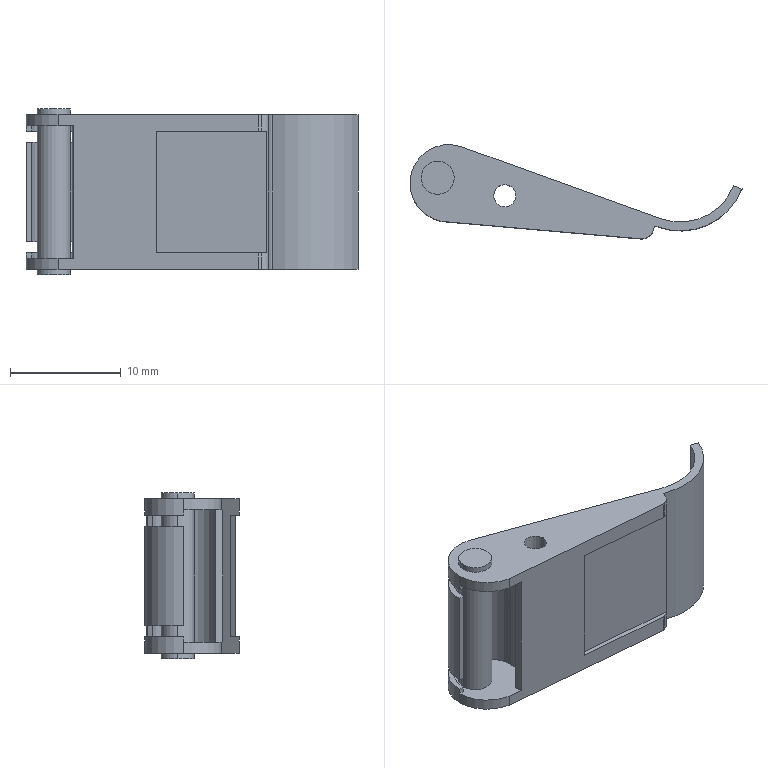Part | SolidWorks | features ICE 6, RefAxis 6, 3DProfileFeature 2, Extrusion 1 | 1 solid | 47 faces | box 30 x 8.531 x 15 mm | volume 1203 mm3 | plane 27 | cylinder 20 | commonest cylinder face diameters 7 x7 3 x6 2 x3 6 x2 10.4 x1 12 x1
STEP:
#1=CARTESIAN_POINT('',(4.,6.,7.5));
#2=VERTEX_POINT('',#1);
#3=CARTESIAN_POINT('',(1.,6.,7.5));
#4=VERTEX_POINT('',#3);
#5=CARTESIAN_POINT('',(2.5,6.,7.5));
#6=DIRECTION('',(0.,0.,1.));
#7=DIRECTION('',(1.,0.,0.));
#8=AXIS2_PLACEMENT_3D('',#5,#6,#7);
#9=CIRCLE('',#8,1.5);
#10=EDGE_CURVE('',#2,#4,#9,.T.);
#11=ORIENTED_EDGE('',*,*,#10,.F.);
#12=CARTESIAN_POINT('',(4.,6.,7.));
#13=VERTEX_POINT('',#12);
#14=CARTESIAN_POINT('',(4.,6.,7.5));
#15=DIRECTION('',(0.,0.,-1.));
#16=VECTOR('',#15,1000.);
#17=LINE('',#14,#16);
#18=EDGE_CURVE('',#2,#13,#17,.T.);
#19=ORIENTED_EDGE('',*,*,#18,.T.);
#20=CARTESIAN_POINT('',(1.,6.,7.));
#21=VERTEX_POINT('',#20);
#22=CARTESIAN_POINT('',(2.5,6.,7.));
#23=DIRECTION('',(0.,0.,-1.));
#24=DIRECTION('',(1.,0.,0.));
#25=AXIS2_PLACEMENT_3D('',#22,#23,#24);
#26=CIRCLE('',#25,1.5);
#27=EDGE_CURVE('',#21,#13,#26,.T.);
#28=ORIENTED_EDGE('',*,*,#27,.F.);
#29=CARTESIAN_POINT('',(1.,6.,7.5));
#30=DIRECTION('',(0.,0.,-1.));
#31=VECTOR('',#30,1000.);
#32=LINE('',#29,#31);
#33=EDGE_CURVE('',#4,#21,#32,.T.);
#34=ORIENTED_EDGE('',*,*,#33,.F.);
#35=EDGE_LOOP('',(#11,#19,#28,#34));
#36=FACE_OUTER_BOUND('',#35,.T.);
#37=CARTESIAN_POINT('',(2.5,6.,7.5));
#38=DIRECTION('',(0.,0.,-1.));
#39=DIRECTION('',(-1.,0.,0.));
#40=AXIS2_PLACEMENT_3D('',#37,#38,#39);
#41=CYLINDRICAL_SURFACE('',#40,1.5);
#42=ADVANCED_FACE('',(#36),#41,.T.);
#43=CARTESIAN_POINT('',(1.,6.,-7.));
#44=VERTEX_POINT('',#43);
#45=CARTESIAN_POINT('',(4.,6.,-7.));
#46=VERTEX_POINT('',#45);
#47=CARTESIAN_POINT('',(2.5,6.,-7.));
#48=DIRECTION('',(0.,0.,-1.));
#49=DIRECTION('',(1.,0.,0.));
#50=AXIS2_PLACEMENT_3D('',#47,#48,#49);
#51=CIRCLE('',#50,1.5);
#52=EDGE_CURVE('',#44,#46,#51,.T.);
#53=ORIENTED_EDGE('',*,*,#52,.T.);
#54=CARTESIAN_POINT('',(4.,6.,-7.5));
#55=VERTEX_POINT('',#54);
#56=CARTESIAN_POINT('',(4.,6.,7.5));
#57=DIRECTION('',(0.,0.,-1.));
#58=VECTOR('',#57,1000.);
#59=LINE('',#56,#58);
#60=EDGE_CURVE('',#46,#55,#59,.T.);
#61=ORIENTED_EDGE('',*,*,#60,.T.);
#62=CARTESIAN_POINT('',(1.,6.,-7.5));
#63=VERTEX_POINT('',#62);
#64=CARTESIAN_POINT('',(2.5,6.,-7.5));
#65=DIRECTION('',(0.,0.,1.));
#66=DIRECTION('',(1.,0.,0.));
#67=AXIS2_PLACEMENT_3D('',#64,#65,#66);
#68=CIRCLE('',#67,1.5);
#69=EDGE_CURVE('',#55,#63,#68,.T.);
#70=ORIENTED_EDGE('',*,*,#69,.T.);
#71=CARTESIAN_POINT('',(1.,6.,7.5));
#72=DIRECTION('',(0.,0.,-1.));
#73=VECTOR('',#72,1000.);
#74=LINE('',#71,#73);
#75=EDGE_CURVE('',#44,#63,#74,.T.);
#76=ORIENTED_EDGE('',*,*,#75,.F.);
#77=EDGE_LOOP('',(#53,#61,#70,#76));
#78=FACE_OUTER_BOUND('',#77,.T.);
#79=CARTESIAN_POINT('',(2.5,6.,7.5));
#80=DIRECTION('',(0.,0.,-1.));
#81=DIRECTION('',(-1.,0.,0.));
#82=AXIS2_PLACEMENT_3D('',#79,#80,#81);
#83=CYLINDRICAL_SURFACE('',#82,1.5);
#84=ADVANCED_FACE('',(#78),#83,.T.);
#85=CARTESIAN_POINT('',(1.,6.,6.));
#86=VERTEX_POINT('',#85);
#87=CARTESIAN_POINT('',(4.,6.,6.));
#88=VERTEX_POINT('',#87);
#89=CARTESIAN_POINT('',(2.5,6.,6.));
#90=DIRECTION('',(0.,0.,-1.));
#91=DIRECTION('',(1.,0.,0.));
#92=AXIS2_PLACEMENT_3D('',#89,#90,#91);
#93=CIRCLE('',#92,1.5);
#94=EDGE_CURVE('',#86,#88,#93,.T.);
#95=ORIENTED_EDGE('',*,*,#94,.T.);
#96=CARTESIAN_POINT('',(4.,6.,-6.));
#97=VERTEX_POINT('',#96);
#98=CARTESIAN_POINT('',(4.,6.,7.5));
#99=DIRECTION('',(0.,0.,-1.));
#100=VECTOR('',#99,1000.);
#101=LINE('',#98,#100);
#102=EDGE_CURVE('',#88,#97,#101,.T.);
#103=ORIENTED_EDGE('',*,*,#102,.T.);
#104=CARTESIAN_POINT('',(1.,6.,-6.));
#105=VERTEX_POINT('',#104);
#106=CARTESIAN_POINT('',(2.5,6.,-6.));
#107=DIRECTION('',(0.,0.,-1.));
#108=DIRECTION('',(1.,0.,0.));
#109=AXIS2_PLACEMENT_3D('',#106,#107,#108);
#110=CIRCLE('',#109,1.5);
#111=EDGE_CURVE('',#105,#97,#110,.T.);
#112=ORIENTED_EDGE('',*,*,#111,.F.);
#113=CARTESIAN_POINT('',(1.,6.,7.5));
#114=DIRECTION('',(0.,0.,-1.));
#115=VECTOR('',#114,1000.);
#116=LINE('',#113,#115);
#117=EDGE_CURVE('',#86,#105,#116,.T.);
#118=ORIENTED_EDGE('',*,*,#117,.F.);
#119=EDGE_LOOP('',(#95,#103,#112,#118));
#120=FACE_OUTER_BOUND('',#119,.T.);
#121=CARTESIAN_POINT('',(2.5,6.,7.5));
#122=DIRECTION('',(0.,0.,-1.));
#123=DIRECTION('',(-1.,0.,0.));
#124=AXIS2_PLACEMENT_3D('',#121,#122,#123);
#125=CYLINDRICAL_SURFACE('',#124,1.5);
#126=ADVANCED_FACE('',(#120),#125,.T.);
#127=CARTESIAN_POINT('',(7.57,4.38,7.));
#128=VERTEX_POINT('',#127);
#129=CARTESIAN_POINT('',(9.57,4.38,7.));
#130=VERTEX_POINT('',#129);
#131=CARTESIAN_POINT('',(8.57,4.38,7.));
#132=DIRECTION('',(0.,0.,1.));
#133=DIRECTION('',(1.,0.,0.));
#134=AXIS2_PLACEMENT_3D('',#131,#132,#133);
#135=CIRCLE('',#134,1.);
#136=EDGE_CURVE('',#128,#130,#135,.T.);
#137=ORIENTED_EDGE('',*,*,#136,.T.);
#138=CARTESIAN_POINT('',(9.57,4.38,-7.));
#139=VERTEX_POINT('',#138);
#140=CARTESIAN_POINT('',(9.57,4.38,7.));
#141=DIRECTION('',(0.,0.,-1.));
#142=VECTOR('',#141,1000.);
#143=LINE('',#140,#142);
#144=EDGE_CURVE('',#130,#139,#143,.T.);
#145=ORIENTED_EDGE('',*,*,#144,.T.);
#146=CARTESIAN_POINT('',(7.57,4.38,-7.));
#147=VERTEX_POINT('',#146);
#148=CARTESIAN_POINT('',(8.57,4.38,-7.));
#149=DIRECTION('',(0.,0.,1.));
#150=DIRECTION('',(1.,0.,0.));
#151=AXIS2_PLACEMENT_3D('',#148,#149,#150);
#152=CIRCLE('',#151,1.);
#153=EDGE_CURVE('',#147,#139,#152,.T.);
#154=ORIENTED_EDGE('',*,*,#153,.F.);
#155=CARTESIAN_POINT('',(7.57,4.38,7.));
#156=DIRECTION('',(0.,0.,-1.));
#157=VECTOR('',#156,1000.);
#158=LINE('',#155,#157);
#159=EDGE_CURVE('',#128,#147,#158,.T.);
#160=ORIENTED_EDGE('',*,*,#159,.F.);
#161=EDGE_LOOP('',(#137,#145,#154,#160));
#162=FACE_OUTER_BOUND('',#161,.T.);
#163=CARTESIAN_POINT('',(8.57,4.38,7.));
#164=DIRECTION('',(0.,0.,-1.));
#165=DIRECTION('',(-1.,0.,0.));
#166=AXIS2_PLACEMENT_3D('',#163,#164,#165);
#167=CYLINDRICAL_SURFACE('',#166,1.);
#168=ADVANCED_FACE('',(#162),#167,.F.);
#169=CARTESIAN_POINT('',(0.,5.5,7.));
#170=VERTEX_POINT('',#169);
#171=CARTESIAN_POINT('',(2.892,2.053,7.));
#172=VERTEX_POINT('',#171);
#173=CARTESIAN_POINT('',(3.5,5.5,7.));
#174=DIRECTION('',(0.,0.,1.));
#175=DIRECTION('',(1.,0.,0.));
#176=AXIS2_PLACEMENT_3D('',#173,#174,#175);
#177=CIRCLE('',#176,3.5);
#178=EDGE_CURVE('',#170,#172,#177,.T.);
#179=ORIENTED_EDGE('',*,*,#178,.F.);
#180=CARTESIAN_POINT('',(0.,5.5,6.));
#181=VERTEX_POINT('',#180);
#182=CARTESIAN_POINT('',(0.,5.5,7.));
#183=DIRECTION('',(0.,0.,-1.));
#184=VECTOR('',#183,1000.);
#185=LINE('',#182,#184);
#186=EDGE_CURVE('',#170,#181,#185,.T.);
#187=ORIENTED_EDGE('',*,*,#186,.T.);
#188=CARTESIAN_POINT('',(2.892,2.053,6.));
#189=VERTEX_POINT('',#188);
#190=CARTESIAN_POINT('',(3.5,5.5,6.));
#191=DIRECTION('',(0.,0.,1.));
#192=DIRECTION('',(1.,0.,0.));
#193=AXIS2_PLACEMENT_3D('',#190,#191,#192);
#194=CIRCLE('',#193,3.5);
#195=EDGE_CURVE('',#181,#189,#194,.T.);
#196=ORIENTED_EDGE('',*,*,#195,.T.);
#197=CARTESIAN_POINT('',(2.892,2.053,7.));
#198=DIRECTION('',(0.,0.,-1.));
#199=VECTOR('',#198,1000.);
#200=LINE('',#197,#199);
#201=EDGE_CURVE('',#172,#189,#200,.T.);
#202=ORIENTED_EDGE('',*,*,#201,.F.);
#203=EDGE_LOOP('',(#179,#187,#196,#202));
#204=FACE_OUTER_BOUND('',#203,.T.);
#205=CARTESIAN_POINT('',(3.5,5.5,7.));
#206=DIRECTION('',(0.,0.,-1.));
#207=DIRECTION('',(-1.,0.,0.));
#208=AXIS2_PLACEMENT_3D('',#205,#206,#207);
#209=CYLINDRICAL_SURFACE('',#208,3.5);
#210=ADVANCED_FACE('',(#204),#209,.T.);
#211=CARTESIAN_POINT('',(6.5,5.5,-6.));
#212=VERTEX_POINT('',#211);
#213=CARTESIAN_POINT('',(0.5,5.5,-6.));
#214=VERTEX_POINT('',#213);
#215=CARTESIAN_POINT('',(3.5,5.5,-6.));
#216=DIRECTION('',(0.,0.,1.));
#217=DIRECTION('',(1.,0.,0.));
#218=AXIS2_PLACEMENT_3D('',#215,#216,#217);
#219=CIRCLE('',#218,3.);
#220=EDGE_CURVE('',#212,#214,#219,.T.);
#221=ORIENTED_EDGE('',*,*,#220,.F.);
#222=CARTESIAN_POINT('',(6.5,5.5,6.));
#223=VERTEX_POINT('',#222);
#224=CARTESIAN_POINT('',(6.5,5.5,-6.));
#225=DIRECTION('',(0.,0.,1.));
#226=VECTOR('',#225,1000.);
#227=LINE('',#224,#226);
#228=EDGE_CURVE('',#212,#223,#227,.T.);
#229=ORIENTED_EDGE('',*,*,#228,.T.);
#230=CARTESIAN_POINT('',(0.5,5.5,6.));
#231=VERTEX_POINT('',#230);
#232=CARTESIAN_POINT('',(3.5,5.5,6.));
#233=DIRECTION('',(0.,0.,1.));
#234=DIRECTION('',(1.,0.,0.));
#235=AXIS2_PLACEMENT_3D('',#232,#233,#234);
#236=CIRCLE('',#235,3.);
#237=EDGE_CURVE('',#223,#231,#236,.T.);
#238=ORIENTED_EDGE('',*,*,#237,.T.);
#239=CARTESIAN_POINT('',(0.5,5.5,5.5));
#240=VERTEX_POINT('',#239);
#241=CARTESIAN_POINT('',(0.5,5.5,-6.));
#242=DIRECTION('',(0.,0.,1.));
#243=VECTOR('',#242,1000.);
#244=LINE('',#241,#243);
#245=EDGE_CURVE('',#240,#231,#244,.T.);
#246=ORIENTED_EDGE('',*,*,#245,.F.);
#247=CARTESIAN_POINT('',(4.526,8.319,5.5));
#248=VERTEX_POINT('',#247);
#249=CARTESIAN_POINT('',(3.5,5.5,5.5));
#250=DIRECTION('',(0.,0.,-1.));
#251=DIRECTION('',(1.,0.,0.));
#252=AXIS2_PLACEMENT_3D('',#249,#250,#251);
#253=CIRCLE('',#252,3.);
#254=EDGE_CURVE('',#240,#248,#253,.T.);
#255=ORIENTED_EDGE('',*,*,#254,.T.);
#256=CARTESIAN_POINT('',(4.526,8.319,4.5));
#257=VERTEX_POINT('',#256);
#258=CARTESIAN_POINT('',(4.526,8.319,-6.));
#259=DIRECTION('',(0.,0.,-1.));
#260=VECTOR('',#259,1000.);
#261=LINE('',#258,#260);
#262=EDGE_CURVE('',#248,#257,#261,.T.);
#263=ORIENTED_EDGE('',*,*,#262,.T.);
#264=CARTESIAN_POINT('',(0.5,5.5,4.5));
#265=VERTEX_POINT('',#264);
#266=CARTESIAN_POINT('',(3.5,5.5,4.5));
#267=DIRECTION('',(0.,0.,-1.));
#268=DIRECTION('',(1.,0.,0.));
#269=AXIS2_PLACEMENT_3D('',#266,#267,#268);
#270=CIRCLE('',#269,3.);
#271=EDGE_CURVE('',#265,#257,#270,.T.);
#272=ORIENTED_EDGE('',*,*,#271,.F.);
#273=CARTESIAN_POINT('',(0.5,5.5,-4.5));
#274=VERTEX_POINT('',#273);
#275=CARTESIAN_POINT('',(0.5,5.5,-6.));
#276=DIRECTION('',(0.,0.,1.));
#277=VECTOR('',#276,1000.);
#278=LINE('',#275,#277);
#279=EDGE_CURVE('',#274,#265,#278,.T.);
#280=ORIENTED_EDGE('',*,*,#279,.F.);
#281=CARTESIAN_POINT('',(4.526,8.319,-4.5));
#282=VERTEX_POINT('',#281);
#283=CARTESIAN_POINT('',(3.5,5.5,-4.5));
#284=DIRECTION('',(0.,0.,-1.));
#285=DIRECTION('',(1.,0.,0.));
#286=AXIS2_PLACEMENT_3D('',#283,#284,#285);
#287=CIRCLE('',#286,3.);
#288=EDGE_CURVE('',#274,#282,#287,.T.);
#289=ORIENTED_EDGE('',*,*,#288,.T.);
#290=CARTESIAN_POINT('',(4.526,8.319,-5.5));
#291=VERTEX_POINT('',#290);
#292=CARTESIAN_POINT('',(4.526,8.319,-6.));
#293=DIRECTION('',(0.,0.,1.));
#294=VECTOR('',#293,1000.);
#295=LINE('',#292,#294);
#296=EDGE_CURVE('',#291,#282,#295,.T.);
#297=ORIENTED_EDGE('',*,*,#296,.F.);
#298=CARTESIAN_POINT('',(0.5,5.5,-5.5));
#299=VERTEX_POINT('',#298);
#300=CARTESIAN_POINT('',(3.5,5.5,-5.5));
#301=DIRECTION('',(0.,0.,-1.));
#302=DIRECTION('',(1.,0.,0.));
#303=AXIS2_PLACEMENT_3D('',#300,#301,#302);
#304=CIRCLE('',#303,3.);
#305=EDGE_CURVE('',#299,#291,#304,.T.);
#306=ORIENTED_EDGE('',*,*,#305,.F.);
#307=CARTESIAN_POINT('',(0.5,5.5,-6.));
#308=DIRECTION('',(0.,0.,1.));
#309=VECTOR('',#308,1000.);
#310=LINE('',#307,#309);
#311=EDGE_CURVE('',#214,#299,#310,.T.);
#312=ORIENTED_EDGE('',*,*,#311,.F.);
#313=EDGE_LOOP('',(#221,#229,#238,#246,#255,#263,#272,#280,#289,#297,#306,#312));
#314=FACE_OUTER_BOUND('',#313,.T.);
#315=CARTESIAN_POINT('',(3.5,5.5,-6.));
#316=DIRECTION('',(0.,0.,1.));
#317=DIRECTION('',(1.,0.,0.));
#318=AXIS2_PLACEMENT_3D('',#315,#316,#317);
#319=CYLINDRICAL_SURFACE('',#318,3.);
#320=ADVANCED_FACE('',(#314),#319,.F.);
#321=CARTESIAN_POINT('',(0.,5.5,-6.));
#322=VERTEX_POINT('',#321);
#323=CARTESIAN_POINT('',(2.892,2.053,-6.));
#324=VERTEX_POINT('',#323);
#325=CARTESIAN_POINT('',(3.5,5.5,-6.));
#326=DIRECTION('',(0.,0.,1.));
#327=DIRECTION('',(1.,0.,0.));
#328=AXIS2_PLACEMENT_3D('',#325,#326,#327);
#329=CIRCLE('',#328,3.5);
#330=EDGE_CURVE('',#322,#324,#329,.T.);
#331=ORIENTED_EDGE('',*,*,#330,.F.);
#332=CARTESIAN_POINT('',(0.,5.5,-7.));
#333=VERTEX_POINT('',#332);
#334=CARTESIAN_POINT('',(0.,5.5,7.));
#335=DIRECTION('',(0.,0.,-1.));
#336=VECTOR('',#335,1000.);
#337=LINE('',#334,#336);
#338=EDGE_CURVE('',#322,#333,#337,.T.);
#339=ORIENTED_EDGE('',*,*,#338,.T.);
#340=CARTESIAN_POINT('',(2.892,2.053,-7.));
#341=VERTEX_POINT('',#340);
#342=CARTESIAN_POINT('',(3.5,5.5,-7.));
#343=DIRECTION('',(0.,0.,1.));
#344=DIRECTION('',(1.,0.,0.));
#345=AXIS2_PLACEMENT_3D('',#342,#343,#344);
#346=CIRCLE('',#345,3.5);
#347=EDGE_CURVE('',#333,#341,#346,.T.);
#348=ORIENTED_EDGE('',*,*,#347,.T.);
#349=CARTESIAN_POINT('',(2.892,2.053,7.));
#350=DIRECTION('',(0.,0.,-1.));
#351=VECTOR('',#350,1000.);
#352=LINE('',#349,#351);
#353=EDGE_CURVE('',#324,#341,#352,.T.);
#354=ORIENTED_EDGE('',*,*,#353,.F.);
#355=EDGE_LOOP('',(#331,#339,#348,#354));
#356=FACE_OUTER_BOUND('',#355,.T.);
#357=CARTESIAN_POINT('',(3.5,5.5,7.));
#358=DIRECTION('',(0.,0.,-1.));
#359=DIRECTION('',(-1.,0.,0.));
#360=AXIS2_PLACEMENT_3D('',#357,#358,#359);
#361=CYLINDRICAL_SURFACE('',#360,3.5);
#362=ADVANCED_FACE('',(#356),#361,.T.);
#363=CARTESIAN_POINT('',(11.748,1.278,-5.5));
#364=VERTEX_POINT('',#363);
#365=CARTESIAN_POINT('',(21.,0.4689,-5.5));
#366=VERTEX_POINT('',#365);
#367=CARTESIAN_POINT('',(2.892,2.053,-5.5));
#368=DIRECTION('',(0.9962,-0.08716,0.));
#369=VECTOR('',#368,1000.);
#370=LINE('',#367,#369);
#371=EDGE_CURVE('',#364,#366,#370,.T.);
#372=ORIENTED_EDGE('',*,*,#371,.F.);
#373=CARTESIAN_POINT('',(11.748,1.278,5.5));
#374=VERTEX_POINT('',#373);
#375=CARTESIAN_POINT('',(11.748,1.278,7.));
#376=DIRECTION('',(0.,0.,1.));
#377=VECTOR('',#376,1000.);
#378=LINE('',#375,#377);
#379=EDGE_CURVE('',#364,#374,#378,.T.);
#380=ORIENTED_EDGE('',*,*,#379,.T.);
#381=CARTESIAN_POINT('',(21.,0.4689,5.5));
#382=VERTEX_POINT('',#381);
#383=CARTESIAN_POINT('',(2.892,2.053,5.5));
#384=DIRECTION('',(0.9962,-0.08716,0.));
#385=VECTOR('',#384,1000.);
#386=LINE('',#383,#385);
#387=EDGE_CURVE('',#374,#382,#386,.T.);
#388=ORIENTED_EDGE('',*,*,#387,.T.);
#389=CARTESIAN_POINT('',(21.,0.4689,7.));
#390=VERTEX_POINT('',#389);
#391=CARTESIAN_POINT('',(21.,0.4689,7.));
#392=DIRECTION('',(0.,0.,-1.));
#393=VECTOR('',#392,1000.);
#394=LINE('',#391,#393);
#395=EDGE_CURVE('',#390,#382,#394,.T.);
#396=ORIENTED_EDGE('',*,*,#395,.F.);
#397=CARTESIAN_POINT('',(2.892,2.053,7.));
#398=DIRECTION('',(0.9962,-0.08716,0.));
#399=VECTOR('',#398,1000.);
#400=LINE('',#397,#399);
#401=EDGE_CURVE('',#172,#390,#400,.T.);
#402=ORIENTED_EDGE('',*,*,#401,.F.);
#403=ORIENTED_EDGE('',*,*,#201,.T.);
#404=CARTESIAN_POINT('',(4.329,1.927,6.));
#405=VERTEX_POINT('',#404);
#406=CARTESIAN_POINT('',(2.892,2.053,6.));
#407=DIRECTION('',(0.9962,-0.08716,0.));
#408=VECTOR('',#407,1000.);
#409=LINE('',#406,#408);
#410=EDGE_CURVE('',#189,#405,#409,.T.);
#411=ORIENTED_EDGE('',*,*,#410,.T.);
#412=CARTESIAN_POINT('',(4.329,1.927,-6.));
#413=VERTEX_POINT('',#412);
#414=CARTESIAN_POINT('',(4.329,1.927,7.));
#415=DIRECTION('',(0.,0.,-1.));
#416=VECTOR('',#415,1000.);
#417=LINE('',#414,#416);
#418=EDGE_CURVE('',#405,#413,#417,.T.);
#419=ORIENTED_EDGE('',*,*,#418,.T.);
#420=CARTESIAN_POINT('',(2.892,2.053,-6.));
#421=DIRECTION('',(0.9962,-0.08716,0.));
#422=VECTOR('',#421,1000.);
#423=LINE('',#420,#422);
#424=EDGE_CURVE('',#324,#413,#423,.T.);
#425=ORIENTED_EDGE('',*,*,#424,.F.);
#426=ORIENTED_EDGE('',*,*,#353,.T.);
#427=CARTESIAN_POINT('',(21.,0.4689,-7.));
#428=VERTEX_POINT('',#427);
#429=CARTESIAN_POINT('',(2.892,2.053,-7.));
#430=DIRECTION('',(0.9962,-0.08716,0.));
#431=VECTOR('',#430,1000.);
#432=LINE('',#429,#431);
#433=EDGE_CURVE('',#341,#428,#432,.T.);
#434=ORIENTED_EDGE('',*,*,#433,.T.);
#435=CARTESIAN_POINT('',(21.,0.4689,7.));
#436=DIRECTION('',(0.,0.,-1.));
#437=VECTOR('',#436,1000.);
#438=LINE('',#435,#437);
#439=EDGE_CURVE('',#366,#428,#438,.T.);
#440=ORIENTED_EDGE('',*,*,#439,.F.);
#441=EDGE_LOOP('',(#372,#380,#388,#396,#402,#403,#411,#419,#425,#426,#434,#440));
#442=FACE_OUTER_BOUND('',#441,.T.);
#443=CARTESIAN_POINT('',(2.892,2.053,7.));
#444=DIRECTION('',(0.08716,0.9962,0.));
#445=DIRECTION('',(-0.9962,0.08716,0.));
#446=AXIS2_PLACEMENT_3D('',#443,#444,#445);
#447=PLANE('',#446);
#448=ADVANCED_FACE('',(#442),#447,.F.);
#449=CARTESIAN_POINT('',(21.244,0.5301,-5.5));
#450=VERTEX_POINT('',#449);
#451=CARTESIAN_POINT('',(21.,0.4689,-5.5));
#452=DIRECTION('',(0.9699,0.2436,0.));
#453=VECTOR('',#452,1000.);
#454=LINE('',#451,#453);
#455=EDGE_CURVE('',#366,#450,#454,.T.);
#456=ORIENTED_EDGE('',*,*,#455,.F.);
#457=ORIENTED_EDGE('',*,*,#439,.T.);
#458=CARTESIAN_POINT('',(21.244,0.5301,-7.));
#459=VERTEX_POINT('',#458);
#460=CARTESIAN_POINT('',(21.,0.4689,-7.));
#461=DIRECTION('',(0.9699,0.2436,0.));
#462=VECTOR('',#461,1000.);
#463=LINE('',#460,#462);
#464=EDGE_CURVE('',#428,#459,#463,.T.);
#465=ORIENTED_EDGE('',*,*,#464,.T.);
#466=CARTESIAN_POINT('',(21.244,0.5301,7.));
#467=DIRECTION('',(0.,0.,-1.));
#468=VECTOR('',#467,1000.);
#469=LINE('',#466,#468);
#470=EDGE_CURVE('',#450,#459,#469,.T.);
#471=ORIENTED_EDGE('',*,*,#470,.F.);
#472=EDGE_LOOP('',(#456,#457,#465,#471));
#473=FACE_OUTER_BOUND('',#472,.T.);
#474=CARTESIAN_POINT('',(21.,0.4689,7.));
#475=DIRECTION('',(-0.2436,0.9699,0.));
#476=DIRECTION('',(-0.9699,-0.2436,0.));
#477=AXIS2_PLACEMENT_3D('',#474,#475,#476);
#478=PLANE('',#477);
#479=ADVANCED_FACE('',(#473),#478,.F.);
#480=CARTESIAN_POINT('',(21.748,0.8362,-5.5));
#481=VERTEX_POINT('',#480);
#482=CARTESIAN_POINT('',(21.,1.5,-5.5));
#483=DIRECTION('',(0.,0.,1.));
#484=DIRECTION('',(1.,0.,0.));
#485=AXIS2_PLACEMENT_3D('',#482,#483,#484);
#486=CIRCLE('',#485,1.);
#487=EDGE_CURVE('',#450,#481,#486,.T.);
#488=ORIENTED_EDGE('',*,*,#487,.F.);
#489=ORIENTED_EDGE('',*,*,#470,.T.);
#490=CARTESIAN_POINT('',(21.928,1.127,-7.));
#491=VERTEX_POINT('',#490);
#492=CARTESIAN_POINT('',(21.,1.5,-7.));
#493=DIRECTION('',(0.,0.,1.));
#494=DIRECTION('',(1.,0.,0.));
#495=AXIS2_PLACEMENT_3D('',#492,#493,#494);
#496=CIRCLE('',#495,1.);
#497=EDGE_CURVE('',#459,#491,#496,.T.);
#498=ORIENTED_EDGE('',*,*,#497,.T.);
#499=CARTESIAN_POINT('',(21.928,1.127,7.));
#500=VERTEX_POINT('',#499);
#501=CARTESIAN_POINT('',(21.928,1.127,7.));
#502=DIRECTION('',(0.,0.,-1.));
#503=VECTOR('',#502,1000.);
#504=LINE('',#501,#503);
#505=EDGE_CURVE('',#500,#491,#504,.T.);
#506=ORIENTED_EDGE('',*,*,#505,.F.);
#507=CARTESIAN_POINT('',(21.244,0.5301,7.));
#508=VERTEX_POINT('',#507);
#509=CARTESIAN_POINT('',(21.,1.5,7.));
#510=DIRECTION('',(0.,0.,1.));
#511=DIRECTION('',(1.,0.,0.));
#512=AXIS2_PLACEMENT_3D('',#509,#510,#511);
#513=CIRCLE('',#512,1.);
#514=EDGE_CURVE('',#508,#500,#513,.T.);
#515=ORIENTED_EDGE('',*,*,#514,.F.);
#516=CARTESIAN_POINT('',(21.244,0.5301,5.5));
#517=VERTEX_POINT('',#516);
#518=CARTESIAN_POINT('',(21.244,0.5301,7.));
#519=DIRECTION('',(0.,0.,-1.));
#520=VECTOR('',#519,1000.);
#521=LINE('',#518,#520);
#522=EDGE_CURVE('',#508,#517,#521,.T.);
#523=ORIENTED_EDGE('',*,*,#522,.T.);
#524=CARTESIAN_POINT('',(21.748,0.8362,5.5));
#525=VERTEX_POINT('',#524);
#526=CARTESIAN_POINT('',(21.,1.5,5.5));
#527=DIRECTION('',(0.,0.,1.));
#528=DIRECTION('',(1.,0.,0.));
#529=AXIS2_PLACEMENT_3D('',#526,#527,#528);
#530=CIRCLE('',#529,1.);
#531=EDGE_CURVE('',#517,#525,#530,.T.);
#532=ORIENTED_EDGE('',*,*,#531,.T.);
#533=CARTESIAN_POINT('',(21.748,0.8362,-5.5));
#534=DIRECTION('',(0.,0.,1.));
#535=VECTOR('',#534,1000.);
#536=LINE('',#533,#535);
#537=EDGE_CURVE('',#481,#525,#536,.T.);
#538=ORIENTED_EDGE('',*,*,#537,.F.);
#539=EDGE_LOOP('',(#488,#489,#498,#506,#515,#523,#532,#538));
#540=FACE_OUTER_BOUND('',#539,.T.);
#541=CARTESIAN_POINT('',(21.,1.5,7.));
#542=DIRECTION('',(0.,0.,-1.));
#543=DIRECTION('',(-1.,0.,0.));
#544=AXIS2_PLACEMENT_3D('',#541,#542,#543);
#545=CYLINDRICAL_SURFACE('',#544,1.);
#546=ADVANCED_FACE('',(#540),#545,.T.);
#547=ORIENTED_EDGE('',*,*,#136,.F.);
#548=CARTESIAN_POINT('',(8.57,4.38,7.));
#549=DIRECTION('',(0.,0.,1.));
#550=DIRECTION('',(1.,0.,0.));
#551=AXIS2_PLACEMENT_3D('',#548,#549,#550);
#552=CIRCLE('',#551,1.);
#553=EDGE_CURVE('',#130,#128,#552,.T.);
#554=ORIENTED_EDGE('',*,*,#553,.F.);
#555=EDGE_LOOP('',(#547,#554));
#556=FACE_BOUND('',#555,.T.);
#557=CARTESIAN_POINT('',(4.688,8.792,7.));
#558=VERTEX_POINT('',#557);
#559=CARTESIAN_POINT('',(3.5,5.5,7.));
#560=DIRECTION('',(0.,0.,1.));
#561=DIRECTION('',(1.,0.,0.));
#562=AXIS2_PLACEMENT_3D('',#559,#560,#561);
#563=CIRCLE('',#562,3.5);
#564=EDGE_CURVE('',#558,#170,#563,.T.);
#565=ORIENTED_EDGE('',*,*,#564,.T.);
#566=ORIENTED_EDGE('',*,*,#178,.T.);
#567=ORIENTED_EDGE('',*,*,#401,.T.);
#568=CARTESIAN_POINT('',(21.,0.4689,7.));
#569=DIRECTION('',(0.9699,0.2436,0.));
#570=VECTOR('',#569,1000.);
#571=LINE('',#568,#570);
#572=EDGE_CURVE('',#390,#508,#571,.T.);
#573=ORIENTED_EDGE('',*,*,#572,.T.);
#574=ORIENTED_EDGE('',*,*,#514,.T.);
#575=CARTESIAN_POINT('',(22.11,1.58,7.));
#576=VERTEX_POINT('',#575);
#577=CARTESIAN_POINT('',(21.928,1.127,7.));
#578=DIRECTION('',(0.3731,0.9278,0.));
#579=VECTOR('',#578,1000.);
#580=LINE('',#577,#579);
#581=EDGE_CURVE('',#500,#576,#580,.T.);
#582=ORIENTED_EDGE('',*,*,#581,.T.);
#583=CARTESIAN_POINT('',(22.319,1.58,7.));
#584=VERTEX_POINT('',#583);
#585=CARTESIAN_POINT('',(22.11,1.58,7.));
#586=DIRECTION('',(1.,0.,0.));
#587=VECTOR('',#586,1000.);
#588=LINE('',#585,#587);
#589=EDGE_CURVE('',#576,#584,#588,.T.);
#590=ORIENTED_EDGE('',*,*,#589,.T.);
#591=CARTESIAN_POINT('',(30.,4.995,7.));
#592=VERTEX_POINT('',#591);
#593=CARTESIAN_POINT('',(24.42,7.2,7.));
#594=DIRECTION('',(0.,0.,1.));
#595=DIRECTION('',(1.,0.,0.));
#596=AXIS2_PLACEMENT_3D('',#593,#594,#595);
#597=CIRCLE('',#596,6.);
#598=EDGE_CURVE('',#584,#592,#597,.T.);
#599=ORIENTED_EDGE('',*,*,#598,.T.);
#600=CARTESIAN_POINT('',(29.248,5.268,7.));
#601=VERTEX_POINT('',#600);
#602=CARTESIAN_POINT('',(30.,4.995,7.));
#603=DIRECTION('',(-0.9397,0.342,0.));
#604=VECTOR('',#603,1000.);
#605=LINE('',#602,#604);
#606=EDGE_CURVE('',#592,#601,#605,.T.);
#607=ORIENTED_EDGE('',*,*,#606,.T.);
#608=CARTESIAN_POINT('',(22.655,2.309,7.));
#609=VERTEX_POINT('',#608);
#610=CARTESIAN_POINT('',(24.42,7.2,7.));
#611=DIRECTION('',(0.,0.,-1.));
#612=DIRECTION('',(-1.,0.,0.));
#613=AXIS2_PLACEMENT_3D('',#610,#611,#612);
#614=CIRCLE('',#613,5.2);
#615=EDGE_CURVE('',#601,#609,#614,.T.);
#616=ORIENTED_EDGE('',*,*,#615,.T.);
#617=CARTESIAN_POINT('',(22.655,2.309,7.));
#618=DIRECTION('',(-0.9406,0.3394,0.));
#619=VECTOR('',#618,1000.);
#620=LINE('',#617,#619);
#621=EDGE_CURVE('',#609,#558,#620,.T.);
#622=ORIENTED_EDGE('',*,*,#621,.T.);
#623=EDGE_LOOP('',(#565,#566,#567,#573,#574,#582,#590,#599,#607,#616,#622));
#624=FACE_OUTER_BOUND('',#623,.T.);
#625=ORIENTED_EDGE('',*,*,#27,.T.);
#626=CARTESIAN_POINT('',(2.5,6.,7.));
#627=DIRECTION('',(0.,0.,-1.));
#628=DIRECTION('',(1.,0.,0.));
#629=AXIS2_PLACEMENT_3D('',#626,#627,#628);
#630=CIRCLE('',#629,1.5);
#631=EDGE_CURVE('',#13,#21,#630,.T.);
#632=ORIENTED_EDGE('',*,*,#631,.T.);
#633=EDGE_LOOP('',(#625,#632));
#634=FACE_BOUND('',#633,.T.);
#635=CARTESIAN_POINT('',(3.5,5.5,7.));
#636=DIRECTION('',(0.,0.,1.));
#637=DIRECTION('',(1.,0.,0.));
#638=AXIS2_PLACEMENT_3D('',#635,#636,#637);
#639=PLANE('',#638);
#640=ADVANCED_FACE('',(#556,#624,#634),#639,.T.);
#641=CARTESIAN_POINT('',(4.688,8.792,-7.));
#642=VERTEX_POINT('',#641);
#643=CARTESIAN_POINT('',(3.5,5.5,-7.));
#644=DIRECTION('',(0.,0.,1.));
#645=DIRECTION('',(1.,0.,0.));
#646=AXIS2_PLACEMENT_3D('',#643,#644,#645);
#647=CIRCLE('',#646,3.5);
#648=EDGE_CURVE('',#642,#333,#647,.T.);
#649=ORIENTED_EDGE('',*,*,#648,.F.);
#650=CARTESIAN_POINT('',(22.655,2.309,-7.));
#651=VERTEX_POINT('',#650);
#652=CARTESIAN_POINT('',(22.655,2.309,-7.));
#653=DIRECTION('',(-0.9406,0.3394,0.));
#654=VECTOR('',#653,1000.);
#655=LINE('',#652,#654);
#656=EDGE_CURVE('',#651,#642,#655,.T.);
#657=ORIENTED_EDGE('',*,*,#656,.F.);
#658=CARTESIAN_POINT('',(29.248,5.268,-7.));
#659=VERTEX_POINT('',#658);
#660=CARTESIAN_POINT('',(24.42,7.2,-7.));
#661=DIRECTION('',(0.,0.,-1.));
#662=DIRECTION('',(-1.,0.,0.));
#663=AXIS2_PLACEMENT_3D('',#660,#661,#662);
#664=CIRCLE('',#663,5.2);
#665=EDGE_CURVE('',#659,#651,#664,.T.);
#666=ORIENTED_EDGE('',*,*,#665,.F.);
#667=CARTESIAN_POINT('',(30.,4.995,-7.));
#668=VERTEX_POINT('',#667);
#669=CARTESIAN_POINT('',(30.,4.995,-7.));
#670=DIRECTION('',(-0.9397,0.342,0.));
#671=VECTOR('',#670,1000.);
#672=LINE('',#669,#671);
#673=EDGE_CURVE('',#668,#659,#672,.T.);
#674=ORIENTED_EDGE('',*,*,#673,.F.);
#675=CARTESIAN_POINT('',(22.319,1.58,-7.));
#676=VERTEX_POINT('',#675);
#677=CARTESIAN_POINT('',(24.42,7.2,-7.));
#678=DIRECTION('',(0.,0.,1.));
#679=DIRECTION('',(1.,0.,0.));
#680=AXIS2_PLACEMENT_3D('',#677,#678,#679);
#681=CIRCLE('',#680,6.);
#682=EDGE_CURVE('',#676,#668,#681,.T.);
#683=ORIENTED_EDGE('',*,*,#682,.F.);
#684=CARTESIAN_POINT('',(22.11,1.58,-7.));
#685=VERTEX_POINT('',#684);
#686=CARTESIAN_POINT('',(22.11,1.58,-7.));
#687=DIRECTION('',(1.,0.,0.));
#688=VECTOR('',#687,1000.);
#689=LINE('',#686,#688);
#690=EDGE_CURVE('',#685,#676,#689,.T.);
#691=ORIENTED_EDGE('',*,*,#690,.F.);
#692=CARTESIAN_POINT('',(21.928,1.127,-7.));
#693=DIRECTION('',(0.3731,0.9278,0.));
#694=VECTOR('',#693,1000.);
#695=LINE('',#692,#694);
#696=EDGE_CURVE('',#491,#685,#695,.T.);
#697=ORIENTED_EDGE('',*,*,#696,.F.);
#698=ORIENTED_EDGE('',*,*,#497,.F.);
#699=ORIENTED_EDGE('',*,*,#464,.F.);
#700=ORIENTED_EDGE('',*,*,#433,.F.);
#701=ORIENTED_EDGE('',*,*,#347,.F.);
#702=EDGE_LOOP('',(#649,#657,#666,#674,#683,#691,#697,#698,#699,#700,#701));
#703=FACE_OUTER_BOUND('',#702,.T.);
#704=ORIENTED_EDGE('',*,*,#153,.T.);
#705=CARTESIAN_POINT('',(8.57,4.38,-7.));
#706=DIRECTION('',(0.,0.,1.));
#707=DIRECTION('',(1.,0.,0.));
#708=AXIS2_PLACEMENT_3D('',#705,#706,#707);
#709=CIRCLE('',#708,1.);
#710=EDGE_CURVE('',#139,#147,#709,.T.);
#711=ORIENTED_EDGE('',*,*,#710,.T.);
#712=EDGE_LOOP('',(#704,#711));
#713=FACE_BOUND('',#712,.T.);
#714=ORIENTED_EDGE('',*,*,#52,.F.);
#715=CARTESIAN_POINT('',(2.5,6.,-7.));
#716=DIRECTION('',(0.,0.,-1.));
#717=DIRECTION('',(1.,0.,0.));
#718=AXIS2_PLACEMENT_3D('',#715,#716,#717);
#719=CIRCLE('',#718,1.5);
#720=EDGE_CURVE('',#46,#44,#719,.T.);
#721=ORIENTED_EDGE('',*,*,#720,.F.);
#722=EDGE_LOOP('',(#714,#721));
#723=FACE_BOUND('',#722,.T.);
#724=CARTESIAN_POINT('',(3.5,5.5,-7.));
#725=DIRECTION('',(0.,0.,1.));
#726=DIRECTION('',(1.,0.,0.));
#727=AXIS2_PLACEMENT_3D('',#724,#725,#726);
#728=PLANE('',#727);
#729=ADVANCED_FACE('',(#703,#713,#723),#728,.F.);
#730=CARTESIAN_POINT('',(4.178,2.578,-6.));
#731=VERTEX_POINT('',#730);
#732=CARTESIAN_POINT('',(3.5,5.5,-6.));
#733=DIRECTION('',(0.,0.,1.));
#734=DIRECTION('',(1.,0.,0.));
#735=AXIS2_PLACEMENT_3D('',#732,#733,#734);
#736=CIRCLE('',#735,3.);
#737=EDGE_CURVE('',#731,#212,#736,.T.);
#738=ORIENTED_EDGE('',*,*,#737,.T.);
#739=ORIENTED_EDGE('',*,*,#220,.T.);
#740=CARTESIAN_POINT('',(3.5,5.5,-6.));
#741=DIRECTION('',(-1.,0.,0.));
#742=VECTOR('',#741,1000.);
#743=LINE('',#740,#742);
#744=EDGE_CURVE('',#214,#322,#743,.T.);
#745=ORIENTED_EDGE('',*,*,#744,.T.);
#746=ORIENTED_EDGE('',*,*,#330,.T.);
#747=ORIENTED_EDGE('',*,*,#424,.T.);
#748=CARTESIAN_POINT('',(4.63,0.6294,-6.));
#749=DIRECTION('',(-0.226,0.9741,0.));
#750=VECTOR('',#749,1000.);
#751=LINE('',#748,#750);
#752=EDGE_CURVE('',#413,#731,#751,.T.);
#753=ORIENTED_EDGE('',*,*,#752,.T.);
#754=EDGE_LOOP('',(#738,#739,#745,#746,#747,#753));
#755=FACE_OUTER_BOUND('',#754,.T.);
#756=ORIENTED_EDGE('',*,*,#111,.T.);
#757=CARTESIAN_POINT('',(2.5,6.,-6.));
#758=DIRECTION('',(0.,0.,-1.));
#759=DIRECTION('',(1.,0.,0.));
#760=AXIS2_PLACEMENT_3D('',#757,#758,#759);
#761=CIRCLE('',#760,1.5);
#762=EDGE_CURVE('',#97,#105,#761,.T.);
#763=ORIENTED_EDGE('',*,*,#762,.T.);
#764=EDGE_LOOP('',(#756,#763));
#765=FACE_BOUND('',#764,.T.);
#766=CARTESIAN_POINT('',(3.5,5.5,-6.));
#767=DIRECTION('',(0.,0.,1.));
#768=DIRECTION('',(1.,0.,0.));
#769=AXIS2_PLACEMENT_3D('',#766,#767,#768);
#770=PLANE('',#769);
#771=ADVANCED_FACE('',(#755,#765),#770,.T.);
#772=CARTESIAN_POINT('',(3.5,5.5,6.));
#773=DIRECTION('',(-1.,0.,0.));
#774=VECTOR('',#773,1000.);
#775=LINE('',#772,#774);
#776=EDGE_CURVE('',#231,#181,#775,.T.);
#777=ORIENTED_EDGE('',*,*,#776,.F.);
#778=ORIENTED_EDGE('',*,*,#237,.F.);
#779=CARTESIAN_POINT('',(4.178,2.578,6.));
#780=VERTEX_POINT('',#779);
#781=CARTESIAN_POINT('',(3.5,5.5,6.));
#782=DIRECTION('',(0.,0.,1.));
#783=DIRECTION('',(1.,0.,0.));
#784=AXIS2_PLACEMENT_3D('',#781,#782,#783);
#785=CIRCLE('',#784,3.);
#786=EDGE_CURVE('',#780,#223,#785,.T.);
#787=ORIENTED_EDGE('',*,*,#786,.F.);
#788=CARTESIAN_POINT('',(4.63,0.6294,6.));
#789=DIRECTION('',(-0.226,0.9741,0.));
#790=VECTOR('',#789,1000.);
#791=LINE('',#788,#790);
#792=EDGE_CURVE('',#405,#780,#791,.T.);
#793=ORIENTED_EDGE('',*,*,#792,.F.);
#794=ORIENTED_EDGE('',*,*,#410,.F.);
#795=ORIENTED_EDGE('',*,*,#195,.F.);
#796=EDGE_LOOP('',(#777,#778,#787,#793,#794,#795));
#797=FACE_OUTER_BOUND('',#796,.T.);
#798=ORIENTED_EDGE('',*,*,#94,.F.);
#799=CARTESIAN_POINT('',(2.5,6.,6.));
#800=DIRECTION('',(0.,0.,-1.));
#801=DIRECTION('',(1.,0.,0.));
#802=AXIS2_PLACEMENT_3D('',#799,#800,#801);
#803=CIRCLE('',#802,1.5);
#804=EDGE_CURVE('',#88,#86,#803,.T.);
#805=ORIENTED_EDGE('',*,*,#804,.F.);
#806=EDGE_LOOP('',(#798,#805));
#807=FACE_BOUND('',#806,.T.);
#808=CARTESIAN_POINT('',(3.5,5.5,6.));
#809=DIRECTION('',(0.,0.,1.));
#810=DIRECTION('',(1.,0.,0.));
#811=AXIS2_PLACEMENT_3D('',#808,#809,#810);
#812=PLANE('',#811);
#813=ADVANCED_FACE('',(#797,#807),#812,.F.);
#814=ORIENTED_EDGE('',*,*,#338,.F.);
#815=CARTESIAN_POINT('',(0.,5.5,-5.5));
#816=VERTEX_POINT('',#815);
#817=CARTESIAN_POINT('',(0.,5.5,7.));
#818=DIRECTION('',(0.,0.,1.));
#819=VECTOR('',#818,1000.);
#820=LINE('',#817,#819);
#821=EDGE_CURVE('',#322,#816,#820,.T.);
#822=ORIENTED_EDGE('',*,*,#821,.T.);
#823=CARTESIAN_POINT('',(4.688,8.792,-5.5));
#824=VERTEX_POINT('',#823);
#825=CARTESIAN_POINT('',(3.5,5.5,-5.5));
#826=DIRECTION('',(0.,0.,1.));
#827=DIRECTION('',(1.,0.,0.));
#828=AXIS2_PLACEMENT_3D('',#825,#826,#827);
#829=CIRCLE('',#828,3.5);
#830=EDGE_CURVE('',#824,#816,#829,.T.);
#831=ORIENTED_EDGE('',*,*,#830,.F.);
#832=CARTESIAN_POINT('',(4.688,8.792,7.));
#833=DIRECTION('',(0.,0.,-1.));
#834=VECTOR('',#833,1000.);
#835=LINE('',#832,#834);
#836=EDGE_CURVE('',#824,#642,#835,.T.);
#837=ORIENTED_EDGE('',*,*,#836,.T.);
#838=ORIENTED_EDGE('',*,*,#648,.T.);
#839=EDGE_LOOP('',(#814,#822,#831,#837,#838));
#840=FACE_OUTER_BOUND('',#839,.T.);
#841=CARTESIAN_POINT('',(3.5,5.5,7.));
#842=DIRECTION('',(0.,0.,-1.));
#843=DIRECTION('',(-1.,0.,0.));
#844=AXIS2_PLACEMENT_3D('',#841,#842,#843);
#845=CYLINDRICAL_SURFACE('',#844,3.5);
#846=ADVANCED_FACE('',(#840),#845,.T.);
#847=CARTESIAN_POINT('',(3.5,5.5,-5.5));
#848=DIRECTION('',(1.,0.,0.));
#849=VECTOR('',#848,1000.);
#850=LINE('',#847,#849);
#851=EDGE_CURVE('',#816,#299,#850,.T.);
#852=ORIENTED_EDGE('',*,*,#851,.F.);
#853=ORIENTED_EDGE('',*,*,#821,.F.);
#854=ORIENTED_EDGE('',*,*,#744,.F.);
#855=ORIENTED_EDGE('',*,*,#311,.T.);
#856=EDGE_LOOP('',(#852,#853,#854,#855));
#857=FACE_OUTER_BOUND('',#856,.T.);
#858=CARTESIAN_POINT('',(3.5,5.5,-6.));
#859=DIRECTION('',(0.,1.,0.));
#860=DIRECTION('',(-1.,0.,0.));
#861=AXIS2_PLACEMENT_3D('',#858,#859,#860);
#862=PLANE('',#861);
#863=ADVANCED_FACE('',(#857),#862,.F.);
#864=CARTESIAN_POINT('',(4.688,8.792,4.5));
#865=VERTEX_POINT('',#864);
#866=CARTESIAN_POINT('',(4.688,8.792,-4.5));
#867=VERTEX_POINT('',#866);
#868=CARTESIAN_POINT('',(4.688,8.792,7.));
#869=DIRECTION('',(0.,0.,-1.));
#870=VECTOR('',#869,1000.);
#871=LINE('',#868,#870);
#872=EDGE_CURVE('',#865,#867,#871,.T.);
#873=ORIENTED_EDGE('',*,*,#872,.T.);
#874=CARTESIAN_POINT('',(0.,5.5,-4.5));
#875=VERTEX_POINT('',#874);
#876=CARTESIAN_POINT('',(3.5,5.5,-4.5));
#877=DIRECTION('',(0.,0.,1.));
#878=DIRECTION('',(1.,0.,0.));
#879=AXIS2_PLACEMENT_3D('',#876,#877,#878);
#880=CIRCLE('',#879,3.5);
#881=EDGE_CURVE('',#867,#875,#880,.T.);
#882=ORIENTED_EDGE('',*,*,#881,.T.);
#883=CARTESIAN_POINT('',(0.,5.5,4.5));
#884=VERTEX_POINT('',#883);
#885=CARTESIAN_POINT('',(0.,5.5,7.));
#886=DIRECTION('',(0.,0.,1.));
#887=VECTOR('',#886,1000.);
#888=LINE('',#885,#887);
#889=EDGE_CURVE('',#875,#884,#888,.T.);
#890=ORIENTED_EDGE('',*,*,#889,.T.);
#891=CARTESIAN_POINT('',(3.5,5.5,4.5));
#892=DIRECTION('',(0.,0.,1.));
#893=DIRECTION('',(1.,0.,0.));
#894=AXIS2_PLACEMENT_3D('',#891,#892,#893);
#895=CIRCLE('',#894,3.5);
#896=EDGE_CURVE('',#865,#884,#895,.T.);
#897=ORIENTED_EDGE('',*,*,#896,.F.);
#898=EDGE_LOOP('',(#873,#882,#890,#897));
#899=FACE_OUTER_BOUND('',#898,.T.);
#900=CARTESIAN_POINT('',(3.5,5.5,7.));
#901=DIRECTION('',(0.,0.,-1.));
#902=DIRECTION('',(-1.,0.,0.));
#903=AXIS2_PLACEMENT_3D('',#900,#901,#902);
#904=CYLINDRICAL_SURFACE('',#903,3.5);
#905=ADVANCED_FACE('',(#899),#904,.T.);
#906=ORIENTED_EDGE('',*,*,#889,.F.);
#907=CARTESIAN_POINT('',(3.5,5.5,-4.5));
#908=DIRECTION('',(1.,0.,0.));
#909=VECTOR('',#908,1000.);
#910=LINE('',#907,#909);
#911=EDGE_CURVE('',#875,#274,#910,.T.);
#912=ORIENTED_EDGE('',*,*,#911,.T.);
#913=ORIENTED_EDGE('',*,*,#279,.T.);
#914=CARTESIAN_POINT('',(3.5,5.5,4.5));
#915=DIRECTION('',(1.,0.,0.));
#916=VECTOR('',#915,1000.);
#917=LINE('',#914,#916);
#918=EDGE_CURVE('',#884,#265,#917,.T.);
#919=ORIENTED_EDGE('',*,*,#918,.F.);
#920=EDGE_LOOP('',(#906,#912,#913,#919));
#921=FACE_OUTER_BOUND('',#920,.T.);
#922=CARTESIAN_POINT('',(3.5,5.5,-6.));
#923=DIRECTION('',(0.,1.,0.));
#924=DIRECTION('',(-1.,0.,0.));
#925=AXIS2_PLACEMENT_3D('',#922,#923,#924);
#926=PLANE('',#925);
#927=ADVANCED_FACE('',(#921),#926,.F.);
#928=ORIENTED_EDGE('',*,*,#228,.F.);
#929=ORIENTED_EDGE('',*,*,#737,.F.);
#930=CARTESIAN_POINT('',(4.178,2.578,-6.));
#931=DIRECTION('',(0.,0.,-1.));
#932=VECTOR('',#931,1000.);
#933=LINE('',#930,#932);
#934=EDGE_CURVE('',#780,#731,#933,.T.);
#935=ORIENTED_EDGE('',*,*,#934,.F.);
#936=ORIENTED_EDGE('',*,*,#786,.T.);
#937=EDGE_LOOP('',(#928,#929,#935,#936));
#938=FACE_OUTER_BOUND('',#937,.T.);
#939=CARTESIAN_POINT('',(3.5,5.5,-6.));
#940=DIRECTION('',(0.,0.,1.));
#941=DIRECTION('',(1.,0.,0.));
#942=AXIS2_PLACEMENT_3D('',#939,#940,#941);
#943=CYLINDRICAL_SURFACE('',#942,3.);
#944=ADVANCED_FACE('',(#938),#943,.F.);
#945=ORIENTED_EDGE('',*,*,#186,.F.);
#946=ORIENTED_EDGE('',*,*,#564,.F.);
#947=CARTESIAN_POINT('',(4.688,8.792,5.5));
#948=VERTEX_POINT('',#947);
#949=CARTESIAN_POINT('',(4.688,8.792,7.));
#950=DIRECTION('',(0.,0.,-1.));
#951=VECTOR('',#950,1000.);
#952=LINE('',#949,#951);
#953=EDGE_CURVE('',#558,#948,#952,.T.);
#954=ORIENTED_EDGE('',*,*,#953,.T.);
#955=CARTESIAN_POINT('',(0.,5.5,5.5));
#956=VERTEX_POINT('',#955);
#957=CARTESIAN_POINT('',(3.5,5.5,5.5));
#958=DIRECTION('',(0.,0.,1.));
#959=DIRECTION('',(1.,0.,0.));
#960=AXIS2_PLACEMENT_3D('',#957,#958,#959);
#961=CIRCLE('',#960,3.5);
#962=EDGE_CURVE('',#948,#956,#961,.T.);
#963=ORIENTED_EDGE('',*,*,#962,.T.);
#964=CARTESIAN_POINT('',(0.,5.5,7.));
#965=DIRECTION('',(0.,0.,1.));
#966=VECTOR('',#965,1000.);
#967=LINE('',#964,#966);
#968=EDGE_CURVE('',#956,#181,#967,.T.);
#969=ORIENTED_EDGE('',*,*,#968,.T.);
#970=EDGE_LOOP('',(#945,#946,#954,#963,#969));
#971=FACE_OUTER_BOUND('',#970,.T.);
#972=CARTESIAN_POINT('',(3.5,5.5,7.));
#973=DIRECTION('',(0.,0.,-1.));
#974=DIRECTION('',(-1.,0.,0.));
#975=AXIS2_PLACEMENT_3D('',#972,#973,#974);
#976=CYLINDRICAL_SURFACE('',#975,3.5);
#977=ADVANCED_FACE('',(#971),#976,.T.);
#978=ORIENTED_EDGE('',*,*,#395,.T.);
#979=CARTESIAN_POINT('',(21.,0.4689,5.5));
#980=DIRECTION('',(0.9699,0.2436,0.));
#981=VECTOR('',#980,1000.);
#982=LINE('',#979,#981);
#983=EDGE_CURVE('',#382,#517,#982,.T.);
#984=ORIENTED_EDGE('',*,*,#983,.T.);
#985=ORIENTED_EDGE('',*,*,#522,.F.);
#986=ORIENTED_EDGE('',*,*,#572,.F.);
#987=EDGE_LOOP('',(#978,#984,#985,#986));
#988=FACE_OUTER_BOUND('',#987,.T.);
#989=CARTESIAN_POINT('',(21.,0.4689,7.));
#990=DIRECTION('',(-0.2436,0.9699,0.));
#991=DIRECTION('',(-0.9699,-0.2436,0.));
#992=AXIS2_PLACEMENT_3D('',#989,#990,#991);
#993=PLANE('',#992);
#994=ADVANCED_FACE('',(#988),#993,.F.);
#995=ORIENTED_EDGE('',*,*,#505,.T.);
#996=ORIENTED_EDGE('',*,*,#696,.T.);
#997=CARTESIAN_POINT('',(22.11,1.58,7.));
#998=DIRECTION('',(0.,0.,-1.));
#999=VECTOR('',#998,1000.);
#1000=LINE('',#997,#999);
#1001=EDGE_CURVE('',#576,#685,#1000,.T.);
#1002=ORIENTED_EDGE('',*,*,#1001,.F.);
#1003=ORIENTED_EDGE('',*,*,#581,.F.);
#1004=EDGE_LOOP('',(#995,#996,#1002,#1003));
#1005=FACE_OUTER_BOUND('',#1004,.T.);
#1006=CARTESIAN_POINT('',(21.928,1.127,7.));
#1007=DIRECTION('',(-0.9278,0.3731,0.));
#1008=DIRECTION('',(-0.3731,-0.9278,0.));
#1009=AXIS2_PLACEMENT_3D('',#1006,#1007,#1008);
#1010=PLANE('',#1009);
#1011=ADVANCED_FACE('',(#1005),#1010,.F.);
#1012=ORIENTED_EDGE('',*,*,#1001,.T.);
#1013=ORIENTED_EDGE('',*,*,#690,.T.);
#1014=CARTESIAN_POINT('',(22.319,1.58,7.));
#1015=DIRECTION('',(0.,0.,-1.));
#1016=VECTOR('',#1015,1000.);
#1017=LINE('',#1014,#1016);
#1018=EDGE_CURVE('',#584,#676,#1017,.T.);
#1019=ORIENTED_EDGE('',*,*,#1018,.F.);
#1020=ORIENTED_EDGE('',*,*,#589,.F.);
#1021=EDGE_LOOP('',(#1012,#1013,#1019,#1020));
#1022=FACE_OUTER_BOUND('',#1021,.T.);
#1023=CARTESIAN_POINT('',(22.11,1.58,7.));
#1024=DIRECTION('',(0.,1.,0.));
#1025=DIRECTION('',(0.,0.,1.));
#1026=AXIS2_PLACEMENT_3D('',#1023,#1024,#1025);
#1027=PLANE('',#1026);
#1028=ADVANCED_FACE('',(#1022),#1027,.F.);
#1029=ORIENTED_EDGE('',*,*,#1018,.T.);
#1030=ORIENTED_EDGE('',*,*,#682,.T.);
#1031=CARTESIAN_POINT('',(30.,4.995,7.));
#1032=DIRECTION('',(0.,0.,-1.));
#1033=VECTOR('',#1032,1000.);
#1034=LINE('',#1031,#1033);
#1035=EDGE_CURVE('',#592,#668,#1034,.T.);
#1036=ORIENTED_EDGE('',*,*,#1035,.F.);
#1037=ORIENTED_EDGE('',*,*,#598,.F.);
#1038=EDGE_LOOP('',(#1029,#1030,#1036,#1037));
#1039=FACE_OUTER_BOUND('',#1038,.T.);
#1040=CARTESIAN_POINT('',(24.42,7.2,7.));
#1041=DIRECTION('',(0.,0.,-1.));
#1042=DIRECTION('',(-1.,0.,0.));
#1043=AXIS2_PLACEMENT_3D('',#1040,#1041,#1042);
#1044=CYLINDRICAL_SURFACE('',#1043,6.);
#1045=ADVANCED_FACE('',(#1039),#1044,.T.);
#1046=ORIENTED_EDGE('',*,*,#1035,.T.);
#1047=ORIENTED_EDGE('',*,*,#673,.T.);
#1048=CARTESIAN_POINT('',(29.248,5.268,7.));
#1049=DIRECTION('',(0.,0.,-1.));
#1050=VECTOR('',#1049,1000.);
#1051=LINE('',#1048,#1050);
#1052=EDGE_CURVE('',#601,#659,#1051,.T.);
#1053=ORIENTED_EDGE('',*,*,#1052,.F.);
#1054=ORIENTED_EDGE('',*,*,#606,.F.);
#1055=EDGE_LOOP('',(#1046,#1047,#1053,#1054));
#1056=FACE_OUTER_BOUND('',#1055,.T.);
#1057=CARTESIAN_POINT('',(30.,4.995,7.));
#1058=DIRECTION('',(-0.342,-0.9397,0.));
#1059=DIRECTION('',(0.9397,-0.342,0.));
#1060=AXIS2_PLACEMENT_3D('',#1057,#1058,#1059);
#1061=PLANE('',#1060);
#1062=ADVANCED_FACE('',(#1056),#1061,.F.);
#1063=ORIENTED_EDGE('',*,*,#1052,.T.);
#1064=ORIENTED_EDGE('',*,*,#665,.T.);
#1065=CARTESIAN_POINT('',(22.655,2.309,7.));
#1066=DIRECTION('',(0.,0.,-1.));
#1067=VECTOR('',#1066,1000.);
#1068=LINE('',#1065,#1067);
#1069=EDGE_CURVE('',#609,#651,#1068,.T.);
#1070=ORIENTED_EDGE('',*,*,#1069,.F.);
#1071=ORIENTED_EDGE('',*,*,#615,.F.);
#1072=EDGE_LOOP('',(#1063,#1064,#1070,#1071));
#1073=FACE_OUTER_BOUND('',#1072,.T.);
#1074=CARTESIAN_POINT('',(24.42,7.2,7.));
#1075=DIRECTION('',(0.,0.,-1.));
#1076=DIRECTION('',(-1.,0.,0.));
#1077=AXIS2_PLACEMENT_3D('',#1074,#1075,#1076);
#1078=CYLINDRICAL_SURFACE('',#1077,5.2);
#1079=ADVANCED_FACE('',(#1073),#1078,.F.);
#1080=ORIENTED_EDGE('',*,*,#1069,.T.);
#1081=ORIENTED_EDGE('',*,*,#656,.T.);
#1082=ORIENTED_EDGE('',*,*,#836,.F.);
#1083=CARTESIAN_POINT('',(4.688,8.792,7.));
#1084=DIRECTION('',(0.,0.,-1.));
#1085=VECTOR('',#1084,1000.);
#1086=LINE('',#1083,#1085);
#1087=EDGE_CURVE('',#867,#824,#1086,.T.);
#1088=ORIENTED_EDGE('',*,*,#1087,.F.);
#1089=ORIENTED_EDGE('',*,*,#872,.F.);
#1090=CARTESIAN_POINT('',(4.688,8.792,4.5));
#1091=DIRECTION('',(0.,0.,1.));
#1092=VECTOR('',#1091,1000.);
#1093=LINE('',#1090,#1092);
#1094=EDGE_CURVE('',#865,#948,#1093,.T.);
#1095=ORIENTED_EDGE('',*,*,#1094,.T.);
#1096=ORIENTED_EDGE('',*,*,#953,.F.);
#1097=ORIENTED_EDGE('',*,*,#621,.F.);
#1098=EDGE_LOOP('',(#1080,#1081,#1082,#1088,#1089,#1095,#1096,#1097));
#1099=FACE_OUTER_BOUND('',#1098,.T.);
#1100=CARTESIAN_POINT('',(22.655,2.309,7.));
#1101=DIRECTION('',(-0.3394,-0.9406,0.));
#1102=DIRECTION('',(0.9406,-0.3394,0.));
#1103=AXIS2_PLACEMENT_3D('',#1100,#1101,#1102);
#1104=PLANE('',#1103);
#1105=ADVANCED_FACE('',(#1099),#1104,.F.);
#1106=ORIENTED_EDGE('',*,*,#144,.F.);
#1107=ORIENTED_EDGE('',*,*,#553,.T.);
#1108=ORIENTED_EDGE('',*,*,#159,.T.);
#1109=ORIENTED_EDGE('',*,*,#710,.F.);
#1110=EDGE_LOOP('',(#1106,#1107,#1108,#1109));
#1111=FACE_OUTER_BOUND('',#1110,.T.);
#1112=CARTESIAN_POINT('',(8.57,4.38,7.));
#1113=DIRECTION('',(0.,0.,-1.));
#1114=DIRECTION('',(-1.,0.,0.));
#1115=AXIS2_PLACEMENT_3D('',#1112,#1113,#1114);
#1116=CYLINDRICAL_SURFACE('',#1115,1.);
#1117=ADVANCED_FACE('',(#1111),#1116,.F.);
#1118=ORIENTED_EDGE('',*,*,#968,.F.);
#1119=CARTESIAN_POINT('',(3.5,5.5,5.5));
#1120=DIRECTION('',(1.,0.,0.));
#1121=VECTOR('',#1120,1000.);
#1122=LINE('',#1119,#1121);
#1123=EDGE_CURVE('',#956,#240,#1122,.T.);
#1124=ORIENTED_EDGE('',*,*,#1123,.T.);
#1125=ORIENTED_EDGE('',*,*,#245,.T.);
#1126=ORIENTED_EDGE('',*,*,#776,.T.);
#1127=EDGE_LOOP('',(#1118,#1124,#1125,#1126));
#1128=FACE_OUTER_BOUND('',#1127,.T.);
#1129=CARTESIAN_POINT('',(3.5,5.5,-6.));
#1130=DIRECTION('',(0.,1.,0.));
#1131=DIRECTION('',(-1.,0.,0.));
#1132=AXIS2_PLACEMENT_3D('',#1129,#1130,#1131);
#1133=PLANE('',#1132);
#1134=ADVANCED_FACE('',(#1128),#1133,.F.);
#1135=ORIENTED_EDGE('',*,*,#792,.T.);
#1136=ORIENTED_EDGE('',*,*,#934,.T.);
#1137=ORIENTED_EDGE('',*,*,#752,.F.);
#1138=ORIENTED_EDGE('',*,*,#418,.F.);
#1139=EDGE_LOOP('',(#1135,#1136,#1137,#1138));
#1140=FACE_OUTER_BOUND('',#1139,.T.);
#1141=CARTESIAN_POINT('',(4.63,0.6294,-6.));
#1142=DIRECTION('',(0.9741,0.226,0.));
#1143=DIRECTION('',(-0.226,0.9741,0.));
#1144=AXIS2_PLACEMENT_3D('',#1141,#1142,#1143);
#1145=PLANE('',#1144);
#1146=ADVANCED_FACE('',(#1140),#1145,.F.);
#1147=CARTESIAN_POINT('',(4.697,8.789,4.5));
#1148=VERTEX_POINT('',#1147);
#1149=CARTESIAN_POINT('',(3.5,5.5,4.5));
#1150=DIRECTION('',(0.,0.,1.));
#1151=DIRECTION('',(1.,0.,0.));
#1152=AXIS2_PLACEMENT_3D('',#1149,#1150,#1151);
#1153=CIRCLE('',#1152,3.5);
#1154=EDGE_CURVE('',#1148,#865,#1153,.T.);
#1155=ORIENTED_EDGE('',*,*,#1154,.F.);
#1156=CARTESIAN_POINT('',(4.697,8.789,5.5));
#1157=VERTEX_POINT('',#1156);
#1158=CARTESIAN_POINT('',(4.697,8.789,4.5));
#1159=DIRECTION('',(0.,0.,1.));
#1160=VECTOR('',#1159,1000.);
#1161=LINE('',#1158,#1160);
#1162=EDGE_CURVE('',#1148,#1157,#1161,.T.);
#1163=ORIENTED_EDGE('',*,*,#1162,.T.);
#1164=CARTESIAN_POINT('',(3.5,5.5,5.5));
#1165=DIRECTION('',(0.,0.,1.));
#1166=DIRECTION('',(1.,0.,0.));
#1167=AXIS2_PLACEMENT_3D('',#1164,#1165,#1166);
#1168=CIRCLE('',#1167,3.5);
#1169=EDGE_CURVE('',#1157,#948,#1168,.T.);
#1170=ORIENTED_EDGE('',*,*,#1169,.T.);
#1171=ORIENTED_EDGE('',*,*,#1094,.F.);
#1172=EDGE_LOOP('',(#1155,#1163,#1170,#1171));
#1173=FACE_OUTER_BOUND('',#1172,.T.);
#1174=CARTESIAN_POINT('',(3.5,5.5,4.5));
#1175=DIRECTION('',(0.,0.,1.));
#1176=DIRECTION('',(1.,0.,0.));
#1177=AXIS2_PLACEMENT_3D('',#1174,#1175,#1176);
#1178=CYLINDRICAL_SURFACE('',#1177,3.5);
#1179=ADVANCED_FACE('',(#1173),#1178,.F.);
#1180=CARTESIAN_POINT('',(2.303,2.211,5.5));
#1181=DIRECTION('',(0.342,0.9397,0.));
#1182=VECTOR('',#1181,1000.);
#1183=LINE('',#1180,#1182);
#1184=EDGE_CURVE('',#248,#1157,#1183,.T.);
#1185=ORIENTED_EDGE('',*,*,#1184,.T.);
#1186=ORIENTED_EDGE('',*,*,#1162,.F.);
#1187=CARTESIAN_POINT('',(2.303,2.211,4.5));
#1188=DIRECTION('',(0.342,0.9397,0.));
#1189=VECTOR('',#1188,1000.);
#1190=LINE('',#1187,#1189);
#1191=EDGE_CURVE('',#257,#1148,#1190,.T.);
#1192=ORIENTED_EDGE('',*,*,#1191,.F.);
#1193=ORIENTED_EDGE('',*,*,#262,.F.);
#1194=EDGE_LOOP('',(#1185,#1186,#1192,#1193));
#1195=FACE_OUTER_BOUND('',#1194,.T.);
#1196=CARTESIAN_POINT('',(2.303,2.211,4.5));
#1197=DIRECTION('',(0.9397,-0.342,0.));
#1198=DIRECTION('',(0.342,0.9397,0.));
#1199=AXIS2_PLACEMENT_3D('',#1196,#1197,#1198);
#1200=PLANE('',#1199);
#1201=ADVANCED_FACE('',(#1195),#1200,.F.);
#1202=ORIENTED_EDGE('',*,*,#918,.T.);
#1203=ORIENTED_EDGE('',*,*,#271,.T.);
#1204=ORIENTED_EDGE('',*,*,#1191,.T.);
#1205=ORIENTED_EDGE('',*,*,#1154,.T.);
#1206=ORIENTED_EDGE('',*,*,#896,.T.);
#1207=EDGE_LOOP('',(#1202,#1203,#1204,#1205,#1206));
#1208=FACE_OUTER_BOUND('',#1207,.T.);
#1209=CARTESIAN_POINT('',(3.5,5.5,4.5));
#1210=DIRECTION('',(0.,0.,1.));
#1211=DIRECTION('',(1.,0.,0.));
#1212=AXIS2_PLACEMENT_3D('',#1209,#1210,#1211);
#1213=PLANE('',#1212);
#1214=ADVANCED_FACE('',(#1208),#1213,.T.);
#1215=ORIENTED_EDGE('',*,*,#962,.F.);
#1216=ORIENTED_EDGE('',*,*,#1169,.F.);
#1217=ORIENTED_EDGE('',*,*,#1184,.F.);
#1218=ORIENTED_EDGE('',*,*,#254,.F.);
#1219=ORIENTED_EDGE('',*,*,#1123,.F.);
#1220=EDGE_LOOP('',(#1215,#1216,#1217,#1218,#1219));
#1221=FACE_OUTER_BOUND('',#1220,.T.);
#1222=CARTESIAN_POINT('',(3.5,5.5,5.5));
#1223=DIRECTION('',(0.,0.,1.));
#1224=DIRECTION('',(1.,0.,0.));
#1225=AXIS2_PLACEMENT_3D('',#1222,#1223,#1224);
#1226=PLANE('',#1225);
#1227=ADVANCED_FACE('',(#1221),#1226,.F.);
#1228=ORIENTED_EDGE('',*,*,#296,.T.);
#1229=CARTESIAN_POINT('',(4.697,8.789,-4.5));
#1230=VERTEX_POINT('',#1229);
#1231=CARTESIAN_POINT('',(2.303,2.211,-4.5));
#1232=DIRECTION('',(0.342,0.9397,0.));
#1233=VECTOR('',#1232,1000.);
#1234=LINE('',#1231,#1233);
#1235=EDGE_CURVE('',#282,#1230,#1234,.T.);
#1236=ORIENTED_EDGE('',*,*,#1235,.T.);
#1237=CARTESIAN_POINT('',(4.697,8.789,-5.5));
#1238=VERTEX_POINT('',#1237);
#1239=CARTESIAN_POINT('',(4.697,8.789,-4.5));
#1240=DIRECTION('',(0.,0.,-1.));
#1241=VECTOR('',#1240,1000.);
#1242=LINE('',#1239,#1241);
#1243=EDGE_CURVE('',#1230,#1238,#1242,.T.);
#1244=ORIENTED_EDGE('',*,*,#1243,.T.);
#1245=CARTESIAN_POINT('',(2.303,2.211,-5.5));
#1246=DIRECTION('',(0.342,0.9397,0.));
#1247=VECTOR('',#1246,1000.);
#1248=LINE('',#1245,#1247);
#1249=EDGE_CURVE('',#291,#1238,#1248,.T.);
#1250=ORIENTED_EDGE('',*,*,#1249,.F.);
#1251=EDGE_LOOP('',(#1228,#1236,#1244,#1250));
#1252=FACE_OUTER_BOUND('',#1251,.T.);
#1253=CARTESIAN_POINT('',(2.303,2.211,-4.5));
#1254=DIRECTION('',(-0.9397,0.342,0.));
#1255=DIRECTION('',(-0.342,-0.9397,0.));
#1256=AXIS2_PLACEMENT_3D('',#1253,#1254,#1255);
#1257=PLANE('',#1256);
#1258=ADVANCED_FACE('',(#1252),#1257,.T.);
#1259=ORIENTED_EDGE('',*,*,#881,.F.);
#1260=CARTESIAN_POINT('',(3.5,5.5,-4.5));
#1261=DIRECTION('',(0.,0.,1.));
#1262=DIRECTION('',(1.,0.,0.));
#1263=AXIS2_PLACEMENT_3D('',#1260,#1261,#1262);
#1264=CIRCLE('',#1263,3.5);
#1265=EDGE_CURVE('',#1230,#867,#1264,.T.);
#1266=ORIENTED_EDGE('',*,*,#1265,.F.);
#1267=ORIENTED_EDGE('',*,*,#1235,.F.);
#1268=ORIENTED_EDGE('',*,*,#288,.F.);
#1269=ORIENTED_EDGE('',*,*,#911,.F.);
#1270=EDGE_LOOP('',(#1259,#1266,#1267,#1268,#1269));
#1271=FACE_OUTER_BOUND('',#1270,.T.);
#1272=CARTESIAN_POINT('',(3.5,5.5,-4.5));
#1273=DIRECTION('',(0.,0.,1.));
#1274=DIRECTION('',(1.,0.,0.));
#1275=AXIS2_PLACEMENT_3D('',#1272,#1273,#1274);
#1276=PLANE('',#1275);
#1277=ADVANCED_FACE('',(#1271),#1276,.F.);
#1278=ORIENTED_EDGE('',*,*,#851,.T.);
#1279=ORIENTED_EDGE('',*,*,#305,.T.);
#1280=ORIENTED_EDGE('',*,*,#1249,.T.);
#1281=CARTESIAN_POINT('',(3.5,5.5,-5.5));
#1282=DIRECTION('',(0.,0.,1.));
#1283=DIRECTION('',(1.,0.,0.));
#1284=AXIS2_PLACEMENT_3D('',#1281,#1282,#1283);
#1285=CIRCLE('',#1284,3.5);
#1286=EDGE_CURVE('',#1238,#824,#1285,.T.);
#1287=ORIENTED_EDGE('',*,*,#1286,.T.);
#1288=ORIENTED_EDGE('',*,*,#830,.T.);
#1289=EDGE_LOOP('',(#1278,#1279,#1280,#1287,#1288));
#1290=FACE_OUTER_BOUND('',#1289,.T.);
#1291=CARTESIAN_POINT('',(3.5,5.5,-5.5));
#1292=DIRECTION('',(0.,0.,1.));
#1293=DIRECTION('',(1.,0.,0.));
#1294=AXIS2_PLACEMENT_3D('',#1291,#1292,#1293);
#1295=PLANE('',#1294);
#1296=ADVANCED_FACE('',(#1290),#1295,.T.);
#1297=ORIENTED_EDGE('',*,*,#1286,.F.);
#1298=ORIENTED_EDGE('',*,*,#1243,.F.);
#1299=ORIENTED_EDGE('',*,*,#1265,.T.);
#1300=ORIENTED_EDGE('',*,*,#1087,.T.);
#1301=EDGE_LOOP('',(#1297,#1298,#1299,#1300));
#1302=FACE_OUTER_BOUND('',#1301,.T.);
#1303=CARTESIAN_POINT('',(3.5,5.5,-4.5));
#1304=DIRECTION('',(0.,0.,-1.));
#1305=DIRECTION('',(-1.,0.,0.));
#1306=AXIS2_PLACEMENT_3D('',#1303,#1304,#1305);
#1307=CYLINDRICAL_SURFACE('',#1306,3.5);
#1308=ADVANCED_FACE('',(#1302),#1307,.F.);
#1309=ORIENTED_EDGE('',*,*,#102,.F.);
#1310=ORIENTED_EDGE('',*,*,#804,.T.);
#1311=ORIENTED_EDGE('',*,*,#117,.T.);
#1312=ORIENTED_EDGE('',*,*,#762,.F.);
#1313=EDGE_LOOP('',(#1309,#1310,#1311,#1312));
#1314=FACE_OUTER_BOUND('',#1313,.T.);
#1315=CARTESIAN_POINT('',(2.5,6.,7.5));
#1316=DIRECTION('',(0.,0.,-1.));
#1317=DIRECTION('',(-1.,0.,0.));
#1318=AXIS2_PLACEMENT_3D('',#1315,#1316,#1317);
#1319=CYLINDRICAL_SURFACE('',#1318,1.5);
#1320=ADVANCED_FACE('',(#1314),#1319,.T.);
#1321=CARTESIAN_POINT('',(2.5,6.,-7.5));
#1322=DIRECTION('',(0.,0.,1.));
#1323=DIRECTION('',(1.,0.,0.));
#1324=AXIS2_PLACEMENT_3D('',#1321,#1322,#1323);
#1325=CIRCLE('',#1324,1.5);
#1326=EDGE_CURVE('',#63,#55,#1325,.T.);
#1327=ORIENTED_EDGE('',*,*,#1326,.F.);
#1328=ORIENTED_EDGE('',*,*,#69,.F.);
#1329=EDGE_LOOP('',(#1327,#1328));
#1330=FACE_OUTER_BOUND('',#1329,.T.);
#1331=CARTESIAN_POINT('',(2.5,6.,-7.5));
#1332=DIRECTION('',(0.,0.,1.));
#1333=DIRECTION('',(1.,0.,0.));
#1334=AXIS2_PLACEMENT_3D('',#1331,#1332,#1333);
#1335=PLANE('',#1334);
#1336=ADVANCED_FACE('',(#1330),#1335,.F.);
#1337=ORIENTED_EDGE('',*,*,#60,.F.);
#1338=ORIENTED_EDGE('',*,*,#720,.T.);
#1339=ORIENTED_EDGE('',*,*,#75,.T.);
#1340=ORIENTED_EDGE('',*,*,#1326,.T.);
#1341=EDGE_LOOP('',(#1337,#1338,#1339,#1340));
#1342=FACE_OUTER_BOUND('',#1341,.T.);
#1343=CARTESIAN_POINT('',(2.5,6.,7.5));
#1344=DIRECTION('',(0.,0.,-1.));
#1345=DIRECTION('',(-1.,0.,0.));
#1346=AXIS2_PLACEMENT_3D('',#1343,#1344,#1345);
#1347=CYLINDRICAL_SURFACE('',#1346,1.5);
#1348=ADVANCED_FACE('',(#1342),#1347,.T.);
#1349=ORIENTED_EDGE('',*,*,#18,.F.);
#1350=CARTESIAN_POINT('',(2.5,6.,7.5));
#1351=DIRECTION('',(0.,0.,1.));
#1352=DIRECTION('',(1.,0.,0.));
#1353=AXIS2_PLACEMENT_3D('',#1350,#1351,#1352);
#1354=CIRCLE('',#1353,1.5);
#1355=EDGE_CURVE('',#4,#2,#1354,.T.);
#1356=ORIENTED_EDGE('',*,*,#1355,.F.);
#1357=ORIENTED_EDGE('',*,*,#33,.T.);
#1358=ORIENTED_EDGE('',*,*,#631,.F.);
#1359=EDGE_LOOP('',(#1349,#1356,#1357,#1358));
#1360=FACE_OUTER_BOUND('',#1359,.T.);
#1361=CARTESIAN_POINT('',(2.5,6.,7.5));
#1362=DIRECTION('',(0.,0.,-1.));
#1363=DIRECTION('',(-1.,0.,0.));
#1364=AXIS2_PLACEMENT_3D('',#1361,#1362,#1363);
#1365=CYLINDRICAL_SURFACE('',#1364,1.5);
#1366=ADVANCED_FACE('',(#1360),#1365,.T.);
#1367=ORIENTED_EDGE('',*,*,#1355,.T.);
#1368=ORIENTED_EDGE('',*,*,#10,.T.);
#1369=EDGE_LOOP('',(#1367,#1368));
#1370=FACE_OUTER_BOUND('',#1369,.T.);
#1371=CARTESIAN_POINT('',(2.5,6.,7.5));
#1372=DIRECTION('',(0.,0.,1.));
#1373=DIRECTION('',(1.,0.,0.));
#1374=AXIS2_PLACEMENT_3D('',#1371,#1372,#1373);
#1375=PLANE('',#1374);
#1376=ADVANCED_FACE('',(#1370),#1375,.T.);
#1377=CARTESIAN_POINT('',(11.786,1.708,-5.5));
#1378=VERTEX_POINT('',#1377);
#1379=CARTESIAN_POINT('',(11.786,1.708,-5.5));
#1380=DIRECTION('',(-0.08716,-0.9962,0.));
#1381=VECTOR('',#1380,1000.);
#1382=LINE('',#1379,#1381);
#1383=EDGE_CURVE('',#1378,#364,#1382,.T.);
#1384=ORIENTED_EDGE('',*,*,#1383,.F.);
#1385=CARTESIAN_POINT('',(11.786,1.708,5.5));
#1386=VERTEX_POINT('',#1385);
#1387=CARTESIAN_POINT('',(11.786,1.708,-5.5));
#1388=DIRECTION('',(0.,0.,1.));
#1389=VECTOR('',#1388,1000.);
#1390=LINE('',#1387,#1389);
#1391=EDGE_CURVE('',#1378,#1386,#1390,.T.);
#1392=ORIENTED_EDGE('',*,*,#1391,.T.);
#1393=CARTESIAN_POINT('',(11.786,1.708,5.5));
#1394=DIRECTION('',(-0.08716,-0.9962,0.));
#1395=VECTOR('',#1394,1000.);
#1396=LINE('',#1393,#1395);
#1397=EDGE_CURVE('',#1386,#374,#1396,.T.);
#1398=ORIENTED_EDGE('',*,*,#1397,.T.);
#1399=ORIENTED_EDGE('',*,*,#379,.F.);
#1400=EDGE_LOOP('',(#1384,#1392,#1398,#1399));
#1401=FACE_OUTER_BOUND('',#1400,.T.);
#1402=CARTESIAN_POINT('',(11.786,1.708,-5.5));
#1403=DIRECTION('',(-0.9962,0.08716,0.));
#1404=DIRECTION('',(-0.08716,-0.9962,0.));
#1405=AXIS2_PLACEMENT_3D('',#1402,#1403,#1404);
#1406=PLANE('',#1405);
#1407=ADVANCED_FACE('',(#1401),#1406,.F.);
#1408=ORIENTED_EDGE('',*,*,#371,.T.);
#1409=ORIENTED_EDGE('',*,*,#455,.T.);
#1410=ORIENTED_EDGE('',*,*,#487,.T.);
#1411=CARTESIAN_POINT('',(21.748,0.8362,-5.5));
#1412=DIRECTION('',(-0.9962,0.08716,0.));
#1413=VECTOR('',#1412,1000.);
#1414=LINE('',#1411,#1413);
#1415=EDGE_CURVE('',#481,#1378,#1414,.T.);
#1416=ORIENTED_EDGE('',*,*,#1415,.T.);
#1417=ORIENTED_EDGE('',*,*,#1383,.T.);
#1418=EDGE_LOOP('',(#1408,#1409,#1410,#1416,#1417));
#1419=FACE_OUTER_BOUND('',#1418,.T.);
#1420=CARTESIAN_POINT('',(0.,0.,-5.5));
#1421=DIRECTION('',(0.,0.,1.));
#1422=DIRECTION('',(1.,0.,0.));
#1423=AXIS2_PLACEMENT_3D('',#1420,#1421,#1422);
#1424=PLANE('',#1423);
#1425=ADVANCED_FACE('',(#1419),#1424,.T.);
#1426=ORIENTED_EDGE('',*,*,#1397,.F.);
#1427=CARTESIAN_POINT('',(21.748,0.8362,5.5));
#1428=DIRECTION('',(-0.9962,0.08716,0.));
#1429=VECTOR('',#1428,1000.);
#1430=LINE('',#1427,#1429);
#1431=EDGE_CURVE('',#525,#1386,#1430,.T.);
#1432=ORIENTED_EDGE('',*,*,#1431,.F.);
#1433=ORIENTED_EDGE('',*,*,#531,.F.);
#1434=ORIENTED_EDGE('',*,*,#983,.F.);
#1435=ORIENTED_EDGE('',*,*,#387,.F.);
#1436=EDGE_LOOP('',(#1426,#1432,#1433,#1434,#1435));
#1437=FACE_OUTER_BOUND('',#1436,.T.);
#1438=CARTESIAN_POINT('',(0.,0.,5.5));
#1439=DIRECTION('',(0.,0.,1.));
#1440=DIRECTION('',(1.,0.,0.));
#1441=AXIS2_PLACEMENT_3D('',#1438,#1439,#1440);
#1442=PLANE('',#1441);
#1443=ADVANCED_FACE('',(#1437),#1442,.F.);
#1444=ORIENTED_EDGE('',*,*,#1391,.F.);
#1445=ORIENTED_EDGE('',*,*,#1415,.F.);
#1446=ORIENTED_EDGE('',*,*,#537,.T.);
#1447=ORIENTED_EDGE('',*,*,#1431,.T.);
#1448=EDGE_LOOP('',(#1444,#1445,#1446,#1447));
#1449=FACE_OUTER_BOUND('',#1448,.T.);
#1450=CARTESIAN_POINT('',(21.748,0.8362,-5.5));
#1451=DIRECTION('',(0.08716,0.9962,0.));
#1452=DIRECTION('',(-0.9962,0.08716,0.));
#1453=AXIS2_PLACEMENT_3D('',#1450,#1451,#1452);
#1454=PLANE('',#1453);
#1455=ADVANCED_FACE('',(#1449),#1454,.F.);
#1456=CLOSED_SHELL('',(#42,#84,#126,#168,#210,#320,#362,#448,#479,#546,#640,#729,#771,#813,#846,#863,#905,#927,#944,#977,#994,#1011,#1028,#1045,#1062,#1079,#1105,#1117,#1134,#1146,#1179,#1201,#1214,#1227,#1258,#1277,#1296,#1308,#1320,#1336,#1348,#1366,#1376,#1407,#1425,#1443,#1455));
#1457=MANIFOLD_SOLID_BREP('',#1456);
#1458=CARTESIAN_POINT('',(0.,0.,0.));
#1459=DIRECTION('',(0.,0.,1.));
#1460=DIRECTION('',(1.,0.,0.));
#1461=AXIS2_PLACEMENT_3D('',#1458,#1459,#1460);
#1462=(LENGTH_UNIT()NAMED_UNIT(*)SI_UNIT(.MILLI.,.METRE.));
#1463=UNCERTAINTY_MEASURE_WITH_UNIT(LENGTH_MEASURE(0.00001),#1462,'','');
#1464=(NAMED_UNIT(*)PLANE_ANGLE_UNIT()SI_UNIT($,.RADIAN.));
#1465=(NAMED_UNIT(*)SI_UNIT($,.STERADIAN.)SOLID_ANGLE_UNIT());
#1466=(GEOMETRIC_REPRESENTATION_CONTEXT(3)GLOBAL_UNCERTAINTY_ASSIGNED_CONTEXT((#1463))GLOBAL_UNIT_ASSIGNED_CONTEXT((#1462,#1464,#1465))REPRESENTATION_CONTEXT('',''));
#1467=ADVANCED_BREP_SHAPE_REPRESENTATION('',(#1457,#1461),#1466);